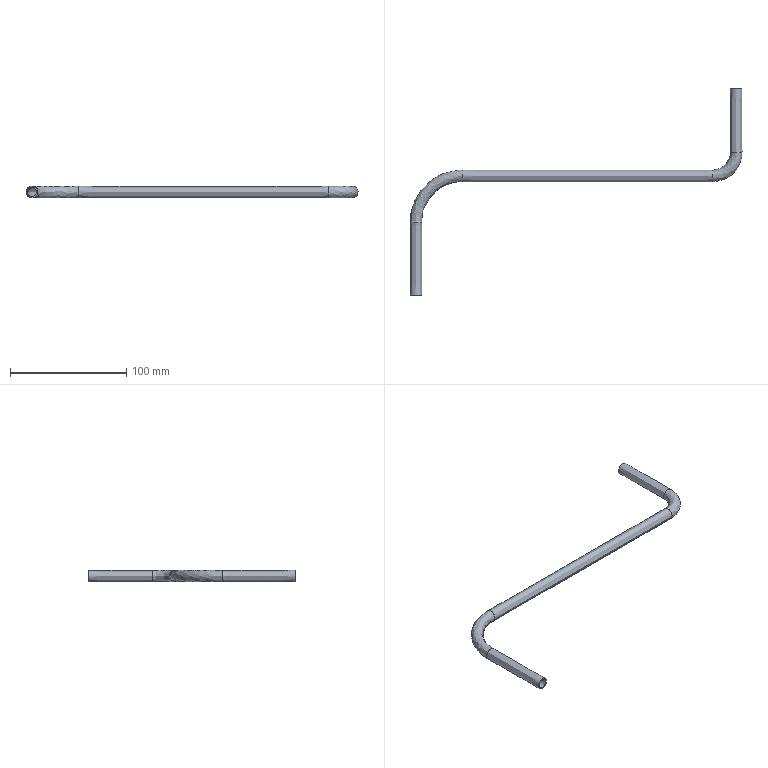Part | NX | features solid 2 | 1 solid | 12 faces | box 285.003 x 177.637 x 10 mm | volume 12073 mm3 | spline 11 | plane 1